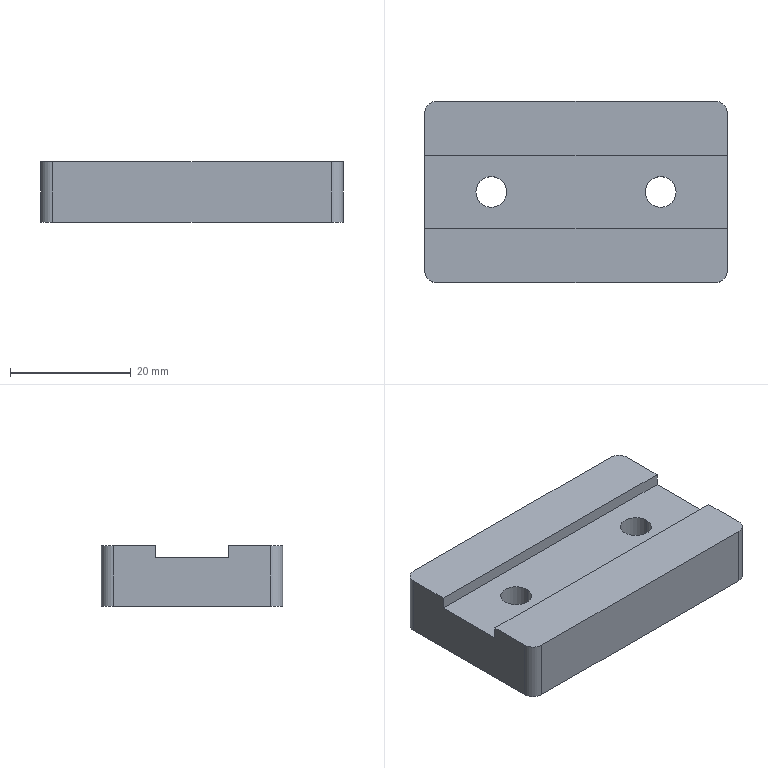Part | STEP file | PN_0044 | 1 solid | 18 faces | box 50 x 30 x 10 mm | volume 13429 mm3 | plane 10 | cylinder 8 | commonest cylinder face diameters 4 x4 5.1 x4
STEP:
#1=CARTESIAN_POINT('',(0.,0.,0.));
#2=DIRECTION('',(0.,0.,1.));
#3=DIRECTION('',(1.,0.,0.));
#4=AXIS2_PLACEMENT_3D('',#1,#2,#3);
#5=CARTESIAN_POINT('',(16.55,0.,0.));
#6=VERTEX_POINT('',#5);
#7=CARTESIAN_POINT('',(16.55,0.,8.));
#8=VERTEX_POINT('',#7);
#9=CARTESIAN_POINT('',(16.55,0.,-7.212));
#10=DIRECTION('',(0.,0.,1.));
#11=VECTOR('',#10,1.);
#12=LINE('',#9,#11);
#13=CARTESIAN_POINT('',(14.,0.,-7.212));
#14=DIRECTION('',(0.,0.,1.));
#15=DIRECTION('',(1.,0.,0.));
#16=AXIS2_PLACEMENT_3D('',#13,#14,#15);
#17=CYLINDRICAL_SURFACE('',#16,2.55);
#18=CARTESIAN_POINT('',(6.283,0.));
#19=DIRECTION('',(0.,1.));
#20=VECTOR('',#19,1.);
#21=LINE('',#18,#20);
#22=(GEOMETRIC_REPRESENTATION_CONTEXT(2)PARAMETRIC_REPRESENTATION_CONTEXT()REPRESENTATION_CONTEXT('',''));
#23=DEFINITIONAL_REPRESENTATION('',(#21),#22);
#24=PCURVE('',#17,#23);
#25=CARTESIAN_POINT('',(14.,0.,-7.212));
#26=DIRECTION('',(0.,0.,1.));
#27=DIRECTION('',(1.,0.,0.));
#28=AXIS2_PLACEMENT_3D('',#25,#26,#27);
#29=CYLINDRICAL_SURFACE('',#28,2.55);
#30=CARTESIAN_POINT('',(0.,0.));
#31=DIRECTION('',(0.,1.));
#32=VECTOR('',#31,1.);
#33=LINE('',#30,#32);
#34=(GEOMETRIC_REPRESENTATION_CONTEXT(2)PARAMETRIC_REPRESENTATION_CONTEXT()REPRESENTATION_CONTEXT('',''));
#35=DEFINITIONAL_REPRESENTATION('',(#33),#34);
#36=PCURVE('',#29,#35);
#37=SURFACE_CURVE('',#12,(#24,#36),.PCURVE_S1.);
#38=EDGE_CURVE('',#6,#8,#37,.T.);
#39=ORIENTED_EDGE('',*,*,#38,.T.);
#40=CARTESIAN_POINT('',(11.45,0.,8.));
#41=VERTEX_POINT('',#40);
#42=CARTESIAN_POINT('',(14.,0.,8.));
#43=DIRECTION('',(0.,0.,1.));
#44=DIRECTION('',(1.,0.,0.));
#45=AXIS2_PLACEMENT_3D('',#42,#43,#44);
#46=CIRCLE('',#45,2.55);
#47=CARTESIAN_POINT('',(0.,15.212));
#48=DIRECTION('',(1.,0.));
#49=VECTOR('',#48,1.);
#50=LINE('',#47,#49);
#51=(GEOMETRIC_REPRESENTATION_CONTEXT(2)PARAMETRIC_REPRESENTATION_CONTEXT()REPRESENTATION_CONTEXT('',''));
#52=DEFINITIONAL_REPRESENTATION('',(#50),#51);
#53=PCURVE('',#17,#52);
#54=CARTESIAN_POINT('',(0.,0.,8.));
#55=DIRECTION('',(0.,0.,-1.));
#56=DIRECTION('',(-1.,0.,0.));
#57=AXIS2_PLACEMENT_3D('',#54,#55,#56);
#58=PLANE('',#57);
#59=CARTESIAN_POINT('',(-16.55,0.));
#60=CARTESIAN_POINT('',(-16.55,4.417));
#61=CARTESIAN_POINT('',(-12.725,2.208));
#62=CARTESIAN_POINT('',(-8.9,0.));
#63=CARTESIAN_POINT('',(-12.725,-2.208));
#64=CARTESIAN_POINT('',(-16.55,-4.417));
#65=CARTESIAN_POINT('',(-16.55,0.));
#66=(BOUNDED_CURVE()B_SPLINE_CURVE(2,(#59,#60,#61,#62,#63,#64,#65),.UNSPECIFIED.,.T.,.F.)B_SPLINE_CURVE_WITH_KNOTS((1,2,2,2,2,1),(-2.094,0.,2.094,4.189,6.283,8.378),.UNSPECIFIED.)CURVE()GEOMETRIC_REPRESENTATION_ITEM()RATIONAL_B_SPLINE_CURVE((1.,0.5,1.,0.5,1.,0.5,1.))REPRESENTATION_ITEM(''));
#67=(GEOMETRIC_REPRESENTATION_CONTEXT(2)PARAMETRIC_REPRESENTATION_CONTEXT()REPRESENTATION_CONTEXT('',''));
#68=DEFINITIONAL_REPRESENTATION('',(#66),#67);
#69=PCURVE('',#58,#68);
#70=SURFACE_CURVE('',#46,(#53,#69),.PCURVE_S1.);
#71=EDGE_CURVE('',#41,#8,#70,.T.);
#72=ORIENTED_EDGE('',*,*,#71,.F.);
#73=CARTESIAN_POINT('',(11.45,0.,0.));
#74=VERTEX_POINT('',#73);
#75=CARTESIAN_POINT('',(11.45,0.,-7.212));
#76=DIRECTION('',(0.,0.,1.));
#77=VECTOR('',#76,1.);
#78=LINE('',#75,#77);
#79=CARTESIAN_POINT('',(3.142,0.));
#80=DIRECTION('',(0.,1.));
#81=VECTOR('',#80,1.);
#82=LINE('',#79,#81);
#83=(GEOMETRIC_REPRESENTATION_CONTEXT(2)PARAMETRIC_REPRESENTATION_CONTEXT()REPRESENTATION_CONTEXT('',''));
#84=DEFINITIONAL_REPRESENTATION('',(#82),#83);
#85=PCURVE('',#17,#84);
#86=CARTESIAN_POINT('',(3.142,0.));
#87=DIRECTION('',(0.,1.));
#88=VECTOR('',#87,1.);
#89=LINE('',#86,#88);
#90=(GEOMETRIC_REPRESENTATION_CONTEXT(2)PARAMETRIC_REPRESENTATION_CONTEXT()REPRESENTATION_CONTEXT('',''));
#91=DEFINITIONAL_REPRESENTATION('',(#89),#90);
#92=PCURVE('',#29,#91);
#93=SURFACE_CURVE('',#78,(#85,#92),.PCURVE_S1.);
#94=EDGE_CURVE('',#74,#41,#93,.T.);
#95=ORIENTED_EDGE('',*,*,#94,.F.);
#96=CARTESIAN_POINT('',(14.,0.,0.));
#97=DIRECTION('',(0.,0.,1.));
#98=DIRECTION('',(-1.,0.,0.));
#99=AXIS2_PLACEMENT_3D('',#96,#97,#98);
#100=CIRCLE('',#99,2.55);
#101=CARTESIAN_POINT('',(3.142,7.212));
#102=DIRECTION('',(1.,0.));
#103=VECTOR('',#102,1.);
#104=LINE('',#101,#103);
#105=(GEOMETRIC_REPRESENTATION_CONTEXT(2)PARAMETRIC_REPRESENTATION_CONTEXT()REPRESENTATION_CONTEXT('',''));
#106=DEFINITIONAL_REPRESENTATION('',(#104),#105);
#107=PCURVE('',#17,#106);
#108=CARTESIAN_POINT('',(0.,0.,0.));
#109=DIRECTION('',(0.,0.,-1.));
#110=DIRECTION('',(-1.,0.,0.));
#111=AXIS2_PLACEMENT_3D('',#108,#109,#110);
#112=PLANE('',#111);
#113=CARTESIAN_POINT('',(-11.45,0.));
#114=CARTESIAN_POINT('',(-11.45,-4.417));
#115=CARTESIAN_POINT('',(-15.275,-2.208));
#116=CARTESIAN_POINT('',(-19.1,0.));
#117=CARTESIAN_POINT('',(-15.275,2.208));
#118=CARTESIAN_POINT('',(-11.45,4.417));
#119=CARTESIAN_POINT('',(-11.45,0.));
#120=(BOUNDED_CURVE()B_SPLINE_CURVE(2,(#113,#114,#115,#116,#117,#118,#119),.UNSPECIFIED.,.T.,.F.)B_SPLINE_CURVE_WITH_KNOTS((1,2,2,2,2,1),(-2.094,0.,2.094,4.189,6.283,8.378),.UNSPECIFIED.)CURVE()GEOMETRIC_REPRESENTATION_ITEM()RATIONAL_B_SPLINE_CURVE((1.,0.5,1.,0.5,1.,0.5,1.))REPRESENTATION_ITEM(''));
#121=(GEOMETRIC_REPRESENTATION_CONTEXT(2)PARAMETRIC_REPRESENTATION_CONTEXT()REPRESENTATION_CONTEXT('',''));
#122=DEFINITIONAL_REPRESENTATION('',(#120),#121);
#123=PCURVE('',#112,#122);
#124=SURFACE_CURVE('',#100,(#107,#123),.PCURVE_S1.);
#125=EDGE_CURVE('',#74,#6,#124,.T.);
#126=ORIENTED_EDGE('',*,*,#125,.T.);
#127=EDGE_LOOP('',(#39,#72,#95,#126));
#128=FACE_BOUND('',#127,.F.);
#129=ADVANCED_FACE('',(#128),#17,.F.);
#130=CARTESIAN_POINT('',(-11.45,0.,0.));
#131=VERTEX_POINT('',#130);
#132=CARTESIAN_POINT('',(-11.45,0.,8.));
#133=VERTEX_POINT('',#132);
#134=CARTESIAN_POINT('',(-11.45,0.,-7.212));
#135=DIRECTION('',(0.,0.,1.));
#136=VECTOR('',#135,1.);
#137=LINE('',#134,#136);
#138=CARTESIAN_POINT('',(-14.,0.,-7.212));
#139=DIRECTION('',(0.,0.,1.));
#140=DIRECTION('',(1.,0.,0.));
#141=AXIS2_PLACEMENT_3D('',#138,#139,#140);
#142=CYLINDRICAL_SURFACE('',#141,2.55);
#143=CARTESIAN_POINT('',(6.283,0.));
#144=DIRECTION('',(0.,1.));
#145=VECTOR('',#144,1.);
#146=LINE('',#143,#145);
#147=(GEOMETRIC_REPRESENTATION_CONTEXT(2)PARAMETRIC_REPRESENTATION_CONTEXT()REPRESENTATION_CONTEXT('',''));
#148=DEFINITIONAL_REPRESENTATION('',(#146),#147);
#149=PCURVE('',#142,#148);
#150=CARTESIAN_POINT('',(-14.,0.,-7.212));
#151=DIRECTION('',(0.,0.,1.));
#152=DIRECTION('',(1.,0.,0.));
#153=AXIS2_PLACEMENT_3D('',#150,#151,#152);
#154=CYLINDRICAL_SURFACE('',#153,2.55);
#155=CARTESIAN_POINT('',(0.,0.));
#156=DIRECTION('',(0.,1.));
#157=VECTOR('',#156,1.);
#158=LINE('',#155,#157);
#159=(GEOMETRIC_REPRESENTATION_CONTEXT(2)PARAMETRIC_REPRESENTATION_CONTEXT()REPRESENTATION_CONTEXT('',''));
#160=DEFINITIONAL_REPRESENTATION('',(#158),#159);
#161=PCURVE('',#154,#160);
#162=SURFACE_CURVE('',#137,(#149,#161),.PCURVE_S1.);
#163=EDGE_CURVE('',#131,#133,#162,.T.);
#164=ORIENTED_EDGE('',*,*,#163,.T.);
#165=CARTESIAN_POINT('',(-16.55,0.,8.));
#166=VERTEX_POINT('',#165);
#167=CARTESIAN_POINT('',(-14.,0.,8.));
#168=DIRECTION('',(0.,0.,1.));
#169=DIRECTION('',(1.,0.,0.));
#170=AXIS2_PLACEMENT_3D('',#167,#168,#169);
#171=CIRCLE('',#170,2.55);
#172=CARTESIAN_POINT('',(0.,15.212));
#173=DIRECTION('',(1.,0.));
#174=VECTOR('',#173,1.);
#175=LINE('',#172,#174);
#176=(GEOMETRIC_REPRESENTATION_CONTEXT(2)PARAMETRIC_REPRESENTATION_CONTEXT()REPRESENTATION_CONTEXT('',''));
#177=DEFINITIONAL_REPRESENTATION('',(#175),#176);
#178=PCURVE('',#142,#177);
#179=CARTESIAN_POINT('',(11.45,0.));
#180=CARTESIAN_POINT('',(11.45,4.417));
#181=CARTESIAN_POINT('',(15.275,2.208));
#182=CARTESIAN_POINT('',(19.1,0.));
#183=CARTESIAN_POINT('',(15.275,-2.208));
#184=CARTESIAN_POINT('',(11.45,-4.417));
#185=CARTESIAN_POINT('',(11.45,0.));
#186=(BOUNDED_CURVE()B_SPLINE_CURVE(2,(#179,#180,#181,#182,#183,#184,#185),.UNSPECIFIED.,.T.,.F.)B_SPLINE_CURVE_WITH_KNOTS((1,2,2,2,2,1),(-2.094,0.,2.094,4.189,6.283,8.378),.UNSPECIFIED.)CURVE()GEOMETRIC_REPRESENTATION_ITEM()RATIONAL_B_SPLINE_CURVE((1.,0.5,1.,0.5,1.,0.5,1.))REPRESENTATION_ITEM(''));
#187=(GEOMETRIC_REPRESENTATION_CONTEXT(2)PARAMETRIC_REPRESENTATION_CONTEXT()REPRESENTATION_CONTEXT('',''));
#188=DEFINITIONAL_REPRESENTATION('',(#186),#187);
#189=PCURVE('',#58,#188);
#190=SURFACE_CURVE('',#171,(#178,#189),.PCURVE_S1.);
#191=EDGE_CURVE('',#166,#133,#190,.T.);
#192=ORIENTED_EDGE('',*,*,#191,.F.);
#193=CARTESIAN_POINT('',(-16.55,0.,0.));
#194=VERTEX_POINT('',#193);
#195=CARTESIAN_POINT('',(-16.55,0.,-7.212));
#196=DIRECTION('',(0.,0.,1.));
#197=VECTOR('',#196,1.);
#198=LINE('',#195,#197);
#199=CARTESIAN_POINT('',(3.142,0.));
#200=DIRECTION('',(0.,1.));
#201=VECTOR('',#200,1.);
#202=LINE('',#199,#201);
#203=(GEOMETRIC_REPRESENTATION_CONTEXT(2)PARAMETRIC_REPRESENTATION_CONTEXT()REPRESENTATION_CONTEXT('',''));
#204=DEFINITIONAL_REPRESENTATION('',(#202),#203);
#205=PCURVE('',#142,#204);
#206=CARTESIAN_POINT('',(3.142,0.));
#207=DIRECTION('',(0.,1.));
#208=VECTOR('',#207,1.);
#209=LINE('',#206,#208);
#210=(GEOMETRIC_REPRESENTATION_CONTEXT(2)PARAMETRIC_REPRESENTATION_CONTEXT()REPRESENTATION_CONTEXT('',''));
#211=DEFINITIONAL_REPRESENTATION('',(#209),#210);
#212=PCURVE('',#154,#211);
#213=SURFACE_CURVE('',#198,(#205,#212),.PCURVE_S1.);
#214=EDGE_CURVE('',#194,#166,#213,.T.);
#215=ORIENTED_EDGE('',*,*,#214,.F.);
#216=CARTESIAN_POINT('',(-14.,0.,0.));
#217=DIRECTION('',(0.,0.,1.));
#218=DIRECTION('',(-1.,0.,0.));
#219=AXIS2_PLACEMENT_3D('',#216,#217,#218);
#220=CIRCLE('',#219,2.55);
#221=CARTESIAN_POINT('',(3.142,7.212));
#222=DIRECTION('',(1.,0.));
#223=VECTOR('',#222,1.);
#224=LINE('',#221,#223);
#225=(GEOMETRIC_REPRESENTATION_CONTEXT(2)PARAMETRIC_REPRESENTATION_CONTEXT()REPRESENTATION_CONTEXT('',''));
#226=DEFINITIONAL_REPRESENTATION('',(#224),#225);
#227=PCURVE('',#142,#226);
#228=CARTESIAN_POINT('',(16.55,0.));
#229=CARTESIAN_POINT('',(16.55,-4.417));
#230=CARTESIAN_POINT('',(12.725,-2.208));
#231=CARTESIAN_POINT('',(8.9,0.));
#232=CARTESIAN_POINT('',(12.725,2.208));
#233=CARTESIAN_POINT('',(16.55,4.417));
#234=CARTESIAN_POINT('',(16.55,0.));
#235=(BOUNDED_CURVE()B_SPLINE_CURVE(2,(#228,#229,#230,#231,#232,#233,#234),.UNSPECIFIED.,.T.,.F.)B_SPLINE_CURVE_WITH_KNOTS((1,2,2,2,2,1),(-2.094,0.,2.094,4.189,6.283,8.378),.UNSPECIFIED.)CURVE()GEOMETRIC_REPRESENTATION_ITEM()RATIONAL_B_SPLINE_CURVE((1.,0.5,1.,0.5,1.,0.5,1.))REPRESENTATION_ITEM(''));
#236=(GEOMETRIC_REPRESENTATION_CONTEXT(2)PARAMETRIC_REPRESENTATION_CONTEXT()REPRESENTATION_CONTEXT('',''));
#237=DEFINITIONAL_REPRESENTATION('',(#235),#236);
#238=PCURVE('',#112,#237);
#239=SURFACE_CURVE('',#220,(#227,#238),.PCURVE_S1.);
#240=EDGE_CURVE('',#194,#131,#239,.T.);
#241=ORIENTED_EDGE('',*,*,#240,.T.);
#242=EDGE_LOOP('',(#164,#192,#215,#241));
#243=FACE_BOUND('',#242,.F.);
#244=ADVANCED_FACE('',(#243),#142,.F.);
#245=CARTESIAN_POINT('',(-25.,-6.05,10.));
#246=VERTEX_POINT('',#245);
#247=CARTESIAN_POINT('',(-25.,-13.,10.));
#248=VERTEX_POINT('',#247);
#249=CARTESIAN_POINT('',(-25.,-15.,10.));
#250=DIRECTION('',(0.,-1.,0.));
#251=VECTOR('',#250,1.);
#252=LINE('',#249,#251);
#253=CARTESIAN_POINT('',(0.,0.,10.));
#254=DIRECTION('',(0.,0.,-1.));
#255=DIRECTION('',(-1.,0.,0.));
#256=AXIS2_PLACEMENT_3D('',#253,#254,#255);
#257=PLANE('',#256);
#258=CARTESIAN_POINT('',(25.,-15.));
#259=DIRECTION('',(0.,-1.));
#260=VECTOR('',#259,1.);
#261=LINE('',#258,#260);
#262=(GEOMETRIC_REPRESENTATION_CONTEXT(2)PARAMETRIC_REPRESENTATION_CONTEXT()REPRESENTATION_CONTEXT('',''));
#263=DEFINITIONAL_REPRESENTATION('',(#261),#262);
#264=PCURVE('',#257,#263);
#265=CARTESIAN_POINT('',(-25.,-15.,10.));
#266=DIRECTION('',(1.,0.,0.));
#267=DIRECTION('',(0.,0.,-1.));
#268=AXIS2_PLACEMENT_3D('',#265,#266,#267);
#269=PLANE('',#268);
#270=CARTESIAN_POINT('',(0.,0.));
#271=DIRECTION('',(0.,-1.));
#272=VECTOR('',#271,1.);
#273=LINE('',#270,#272);
#274=(GEOMETRIC_REPRESENTATION_CONTEXT(2)PARAMETRIC_REPRESENTATION_CONTEXT()REPRESENTATION_CONTEXT('',''));
#275=DEFINITIONAL_REPRESENTATION('',(#273),#274);
#276=PCURVE('',#269,#275);
#277=SURFACE_CURVE('',#252,(#264,#276),.PCURVE_S1.);
#278=EDGE_CURVE('',#246,#248,#277,.T.);
#279=ORIENTED_EDGE('',*,*,#278,.T.);
#280=CARTESIAN_POINT('',(-23.,-15.,10.));
#281=VERTEX_POINT('',#280);
#282=CARTESIAN_POINT('',(-23.,-13.,10.));
#283=DIRECTION('',(0.,0.,1.));
#284=DIRECTION('',(-1.,0.,0.));
#285=AXIS2_PLACEMENT_3D('',#282,#283,#284);
#286=CIRCLE('',#285,2.);
#287=CARTESIAN_POINT('',(25.,-13.));
#288=CARTESIAN_POINT('',(25.,-16.464));
#289=CARTESIAN_POINT('',(22.,-14.732));
#290=CARTESIAN_POINT('',(19.,-13.));
#291=CARTESIAN_POINT('',(22.,-11.268));
#292=CARTESIAN_POINT('',(25.,-9.536));
#293=CARTESIAN_POINT('',(25.,-13.));
#294=(BOUNDED_CURVE()B_SPLINE_CURVE(2,(#287,#288,#289,#290,#291,#292,#293),.UNSPECIFIED.,.T.,.F.)B_SPLINE_CURVE_WITH_KNOTS((1,2,2,2,2,1),(-2.094,0.,2.094,4.189,6.283,8.378),.UNSPECIFIED.)CURVE()GEOMETRIC_REPRESENTATION_ITEM()RATIONAL_B_SPLINE_CURVE((1.,0.5,1.,0.5,1.,0.5,1.))REPRESENTATION_ITEM(''));
#295=(GEOMETRIC_REPRESENTATION_CONTEXT(2)PARAMETRIC_REPRESENTATION_CONTEXT()REPRESENTATION_CONTEXT('',''));
#296=DEFINITIONAL_REPRESENTATION('',(#294),#295);
#297=PCURVE('',#257,#296);
#298=CARTESIAN_POINT('',(-23.,-13.,10.));
#299=DIRECTION('',(0.,0.,-1.));
#300=DIRECTION('',(-1.,0.,0.));
#301=AXIS2_PLACEMENT_3D('',#298,#299,#300);
#302=CYLINDRICAL_SURFACE('',#301,2.);
#303=CARTESIAN_POINT('',(6.283,0.));
#304=DIRECTION('',(-1.,0.));
#305=VECTOR('',#304,1.);
#306=LINE('',#303,#305);
#307=(GEOMETRIC_REPRESENTATION_CONTEXT(2)PARAMETRIC_REPRESENTATION_CONTEXT()REPRESENTATION_CONTEXT('',''));
#308=DEFINITIONAL_REPRESENTATION('',(#306),#307);
#309=PCURVE('',#302,#308);
#310=SURFACE_CURVE('',#286,(#297,#309),.PCURVE_S1.);
#311=EDGE_CURVE('',#248,#281,#310,.T.);
#312=ORIENTED_EDGE('',*,*,#311,.T.);
#313=CARTESIAN_POINT('',(23.,-15.,10.));
#314=VERTEX_POINT('',#313);
#315=CARTESIAN_POINT('',(-25.,-15.,10.));
#316=DIRECTION('',(1.,0.,0.));
#317=VECTOR('',#316,1.);
#318=LINE('',#315,#317);
#319=CARTESIAN_POINT('',(25.,-15.));
#320=DIRECTION('',(-1.,0.));
#321=VECTOR('',#320,1.);
#322=LINE('',#319,#321);
#323=(GEOMETRIC_REPRESENTATION_CONTEXT(2)PARAMETRIC_REPRESENTATION_CONTEXT()REPRESENTATION_CONTEXT('',''));
#324=DEFINITIONAL_REPRESENTATION('',(#322),#323);
#325=PCURVE('',#257,#324);
#326=CARTESIAN_POINT('',(-25.,-15.,10.));
#327=DIRECTION('',(0.,1.,0.));
#328=DIRECTION('',(0.,0.,1.));
#329=AXIS2_PLACEMENT_3D('',#326,#327,#328);
#330=PLANE('',#329);
#331=CARTESIAN_POINT('',(0.,0.));
#332=DIRECTION('',(0.,1.));
#333=VECTOR('',#332,1.);
#334=LINE('',#331,#333);
#335=(GEOMETRIC_REPRESENTATION_CONTEXT(2)PARAMETRIC_REPRESENTATION_CONTEXT()REPRESENTATION_CONTEXT('',''));
#336=DEFINITIONAL_REPRESENTATION('',(#334),#335);
#337=PCURVE('',#330,#336);
#338=SURFACE_CURVE('',#318,(#325,#337),.PCURVE_S1.);
#339=EDGE_CURVE('',#281,#314,#338,.T.);
#340=ORIENTED_EDGE('',*,*,#339,.T.);
#341=CARTESIAN_POINT('',(25.,-13.,10.));
#342=VERTEX_POINT('',#341);
#343=CARTESIAN_POINT('',(23.,-13.,10.));
#344=DIRECTION('',(0.,0.,1.));
#345=DIRECTION('',(-1.,0.,0.));
#346=AXIS2_PLACEMENT_3D('',#343,#344,#345);
#347=CIRCLE('',#346,2.);
#348=CARTESIAN_POINT('',(-21.,-13.));
#349=CARTESIAN_POINT('',(-21.,-16.464));
#350=CARTESIAN_POINT('',(-24.,-14.732));
#351=CARTESIAN_POINT('',(-27.,-13.));
#352=CARTESIAN_POINT('',(-24.,-11.268));
#353=CARTESIAN_POINT('',(-21.,-9.536));
#354=CARTESIAN_POINT('',(-21.,-13.));
#355=(BOUNDED_CURVE()B_SPLINE_CURVE(2,(#348,#349,#350,#351,#352,#353,#354),.UNSPECIFIED.,.T.,.F.)B_SPLINE_CURVE_WITH_KNOTS((1,2,2,2,2,1),(-2.094,0.,2.094,4.189,6.283,8.378),.UNSPECIFIED.)CURVE()GEOMETRIC_REPRESENTATION_ITEM()RATIONAL_B_SPLINE_CURVE((1.,0.5,1.,0.5,1.,0.5,1.))REPRESENTATION_ITEM(''));
#356=(GEOMETRIC_REPRESENTATION_CONTEXT(2)PARAMETRIC_REPRESENTATION_CONTEXT()REPRESENTATION_CONTEXT('',''));
#357=DEFINITIONAL_REPRESENTATION('',(#355),#356);
#358=PCURVE('',#257,#357);
#359=CARTESIAN_POINT('',(23.,-13.,10.));
#360=DIRECTION('',(0.,0.,-1.));
#361=DIRECTION('',(-1.,0.,0.));
#362=AXIS2_PLACEMENT_3D('',#359,#360,#361);
#363=CYLINDRICAL_SURFACE('',#362,2.);
#364=CARTESIAN_POINT('',(6.283,0.));
#365=DIRECTION('',(-1.,0.));
#366=VECTOR('',#365,1.);
#367=LINE('',#364,#366);
#368=(GEOMETRIC_REPRESENTATION_CONTEXT(2)PARAMETRIC_REPRESENTATION_CONTEXT()REPRESENTATION_CONTEXT('',''));
#369=DEFINITIONAL_REPRESENTATION('',(#367),#368);
#370=PCURVE('',#363,#369);
#371=SURFACE_CURVE('',#347,(#358,#370),.PCURVE_S1.);
#372=EDGE_CURVE('',#314,#342,#371,.T.);
#373=ORIENTED_EDGE('',*,*,#372,.T.);
#374=CARTESIAN_POINT('',(25.,-6.05,10.));
#375=VERTEX_POINT('',#374);
#376=CARTESIAN_POINT('',(25.,-15.,10.));
#377=DIRECTION('',(0.,1.,0.));
#378=VECTOR('',#377,1.);
#379=LINE('',#376,#378);
#380=CARTESIAN_POINT('',(-25.,-15.));
#381=DIRECTION('',(0.,1.));
#382=VECTOR('',#381,1.);
#383=LINE('',#380,#382);
#384=(GEOMETRIC_REPRESENTATION_CONTEXT(2)PARAMETRIC_REPRESENTATION_CONTEXT()REPRESENTATION_CONTEXT('',''));
#385=DEFINITIONAL_REPRESENTATION('',(#383),#384);
#386=PCURVE('',#257,#385);
#387=CARTESIAN_POINT('',(25.,-15.,10.));
#388=DIRECTION('',(-1.,0.,0.));
#389=DIRECTION('',(0.,0.,1.));
#390=AXIS2_PLACEMENT_3D('',#387,#388,#389);
#391=PLANE('',#390);
#392=CARTESIAN_POINT('',(0.,0.));
#393=DIRECTION('',(0.,1.));
#394=VECTOR('',#393,1.);
#395=LINE('',#392,#394);
#396=(GEOMETRIC_REPRESENTATION_CONTEXT(2)PARAMETRIC_REPRESENTATION_CONTEXT()REPRESENTATION_CONTEXT('',''));
#397=DEFINITIONAL_REPRESENTATION('',(#395),#396);
#398=PCURVE('',#391,#397);
#399=SURFACE_CURVE('',#379,(#386,#398),.PCURVE_S1.);
#400=EDGE_CURVE('',#342,#375,#399,.T.);
#401=ORIENTED_EDGE('',*,*,#400,.T.);
#402=CARTESIAN_POINT('',(0.,-6.05,10.));
#403=DIRECTION('',(-1.,0.,0.));
#404=VECTOR('',#403,1.);
#405=LINE('',#402,#404);
#406=CARTESIAN_POINT('',(0.,-6.05));
#407=DIRECTION('',(1.,0.));
#408=VECTOR('',#407,1.);
#409=LINE('',#406,#408);
#410=(GEOMETRIC_REPRESENTATION_CONTEXT(2)PARAMETRIC_REPRESENTATION_CONTEXT()REPRESENTATION_CONTEXT('',''));
#411=DEFINITIONAL_REPRESENTATION('',(#409),#410);
#412=PCURVE('',#257,#411);
#413=CARTESIAN_POINT('',(-30.,-6.05,8.));
#414=DIRECTION('',(0.,-1.,0.));
#415=DIRECTION('',(0.,0.,-1.));
#416=AXIS2_PLACEMENT_3D('',#413,#414,#415);
#417=PLANE('',#416);
#418=CARTESIAN_POINT('',(-2.,30.));
#419=DIRECTION('',(0.,-1.));
#420=VECTOR('',#419,1.);
#421=LINE('',#418,#420);
#422=(GEOMETRIC_REPRESENTATION_CONTEXT(2)PARAMETRIC_REPRESENTATION_CONTEXT()REPRESENTATION_CONTEXT('',''));
#423=DEFINITIONAL_REPRESENTATION('',(#421),#422);
#424=PCURVE('',#417,#423);
#425=SURFACE_CURVE('',#405,(#412,#424),.PCURVE_S1.);
#426=EDGE_CURVE('',#375,#246,#425,.T.);
#427=ORIENTED_EDGE('',*,*,#426,.T.);
#428=EDGE_LOOP('',(#279,#312,#340,#373,#401,#427));
#429=FACE_BOUND('',#428,.T.);
#430=ADVANCED_FACE('',(#429),#257,.F.);
#431=ORIENTED_EDGE('',*,*,#400,.F.);
#432=CARTESIAN_POINT('',(25.,-13.,0.));
#433=VERTEX_POINT('',#432);
#434=CARTESIAN_POINT('',(25.,-13.,10.));
#435=DIRECTION('',(0.,0.,-1.));
#436=VECTOR('',#435,1.);
#437=LINE('',#434,#436);
#438=CARTESIAN_POINT('',(0.,2.));
#439=DIRECTION('',(-1.,0.));
#440=VECTOR('',#439,1.);
#441=LINE('',#438,#440);
#442=(GEOMETRIC_REPRESENTATION_CONTEXT(2)PARAMETRIC_REPRESENTATION_CONTEXT()REPRESENTATION_CONTEXT('',''));
#443=DEFINITIONAL_REPRESENTATION('',(#441),#442);
#444=PCURVE('',#391,#443);
#445=CARTESIAN_POINT('',(3.142,0.));
#446=DIRECTION('',(0.,1.));
#447=VECTOR('',#446,1.);
#448=LINE('',#445,#447);
#449=(GEOMETRIC_REPRESENTATION_CONTEXT(2)PARAMETRIC_REPRESENTATION_CONTEXT()REPRESENTATION_CONTEXT('',''));
#450=DEFINITIONAL_REPRESENTATION('',(#448),#449);
#451=PCURVE('',#363,#450);
#452=SURFACE_CURVE('',#437,(#444,#451),.PCURVE_S1.);
#453=EDGE_CURVE('',#342,#433,#452,.T.);
#454=ORIENTED_EDGE('',*,*,#453,.T.);
#455=CARTESIAN_POINT('',(25.,13.,0.));
#456=VERTEX_POINT('',#455);
#457=CARTESIAN_POINT('',(25.,-15.,0.));
#458=DIRECTION('',(0.,1.,0.));
#459=VECTOR('',#458,1.);
#460=LINE('',#457,#459);
#461=CARTESIAN_POINT('',(-10.,0.));
#462=DIRECTION('',(0.,1.));
#463=VECTOR('',#462,1.);
#464=LINE('',#461,#463);
#465=(GEOMETRIC_REPRESENTATION_CONTEXT(2)PARAMETRIC_REPRESENTATION_CONTEXT()REPRESENTATION_CONTEXT('',''));
#466=DEFINITIONAL_REPRESENTATION('',(#464),#465);
#467=PCURVE('',#391,#466);
#468=CARTESIAN_POINT('',(-25.,-15.));
#469=DIRECTION('',(0.,1.));
#470=VECTOR('',#469,1.);
#471=LINE('',#468,#470);
#472=(GEOMETRIC_REPRESENTATION_CONTEXT(2)PARAMETRIC_REPRESENTATION_CONTEXT()REPRESENTATION_CONTEXT('',''));
#473=DEFINITIONAL_REPRESENTATION('',(#471),#472);
#474=PCURVE('',#112,#473);
#475=SURFACE_CURVE('',#460,(#467,#474),.PCURVE_S1.);
#476=EDGE_CURVE('',#433,#456,#475,.T.);
#477=ORIENTED_EDGE('',*,*,#476,.T.);
#478=CARTESIAN_POINT('',(25.,13.,10.));
#479=VERTEX_POINT('',#478);
#480=CARTESIAN_POINT('',(25.,13.,10.));
#481=DIRECTION('',(0.,0.,1.));
#482=VECTOR('',#481,1.);
#483=LINE('',#480,#482);
#484=CARTESIAN_POINT('',(0.,28.));
#485=DIRECTION('',(1.,0.));
#486=VECTOR('',#485,1.);
#487=LINE('',#484,#486);
#488=(GEOMETRIC_REPRESENTATION_CONTEXT(2)PARAMETRIC_REPRESENTATION_CONTEXT()REPRESENTATION_CONTEXT('',''));
#489=DEFINITIONAL_REPRESENTATION('',(#487),#488);
#490=PCURVE('',#391,#489);
#491=CARTESIAN_POINT('',(23.,13.,10.));
#492=DIRECTION('',(0.,0.,-1.));
#493=DIRECTION('',(-1.,0.,0.));
#494=AXIS2_PLACEMENT_3D('',#491,#492,#493);
#495=CYLINDRICAL_SURFACE('',#494,2.);
#496=CARTESIAN_POINT('',(3.142,0.));
#497=DIRECTION('',(0.,-1.));
#498=VECTOR('',#497,1.);
#499=LINE('',#496,#498);
#500=(GEOMETRIC_REPRESENTATION_CONTEXT(2)PARAMETRIC_REPRESENTATION_CONTEXT()REPRESENTATION_CONTEXT('',''));
#501=DEFINITIONAL_REPRESENTATION('',(#499),#500);
#502=PCURVE('',#495,#501);
#503=SURFACE_CURVE('',#483,(#490,#502),.PCURVE_S1.);
#504=EDGE_CURVE('',#456,#479,#503,.T.);
#505=ORIENTED_EDGE('',*,*,#504,.T.);
#506=CARTESIAN_POINT('',(25.,6.05,10.));
#507=VERTEX_POINT('',#506);
#508=CARTESIAN_POINT('',(25.,-15.,10.));
#509=DIRECTION('',(0.,1.,0.));
#510=VECTOR('',#509,1.);
#511=LINE('',#508,#510);
#512=CARTESIAN_POINT('',(0.,0.));
#513=DIRECTION('',(0.,1.));
#514=VECTOR('',#513,1.);
#515=LINE('',#512,#514);
#516=(GEOMETRIC_REPRESENTATION_CONTEXT(2)PARAMETRIC_REPRESENTATION_CONTEXT()REPRESENTATION_CONTEXT('',''));
#517=DEFINITIONAL_REPRESENTATION('',(#515),#516);
#518=PCURVE('',#391,#517);
#519=CARTESIAN_POINT('',(0.,0.,10.));
#520=DIRECTION('',(0.,0.,-1.));
#521=DIRECTION('',(-1.,0.,0.));
#522=AXIS2_PLACEMENT_3D('',#519,#520,#521);
#523=PLANE('',#522);
#524=CARTESIAN_POINT('',(-25.,-15.));
#525=DIRECTION('',(0.,1.));
#526=VECTOR('',#525,1.);
#527=LINE('',#524,#526);
#528=(GEOMETRIC_REPRESENTATION_CONTEXT(2)PARAMETRIC_REPRESENTATION_CONTEXT()REPRESENTATION_CONTEXT('',''));
#529=DEFINITIONAL_REPRESENTATION('',(#527),#528);
#530=PCURVE('',#523,#529);
#531=SURFACE_CURVE('',#511,(#518,#530),.PCURVE_S1.);
#532=EDGE_CURVE('',#507,#479,#531,.T.);
#533=ORIENTED_EDGE('',*,*,#532,.F.);
#534=CARTESIAN_POINT('',(25.,6.05,8.));
#535=VERTEX_POINT('',#534);
#536=CARTESIAN_POINT('',(25.,6.05,10.));
#537=DIRECTION('',(0.,0.,-1.));
#538=VECTOR('',#537,1.);
#539=LINE('',#536,#538);
#540=CARTESIAN_POINT('',(0.,21.05));
#541=DIRECTION('',(-1.,0.));
#542=VECTOR('',#541,1.);
#543=LINE('',#540,#542);
#544=(GEOMETRIC_REPRESENTATION_CONTEXT(2)PARAMETRIC_REPRESENTATION_CONTEXT()REPRESENTATION_CONTEXT('',''));
#545=DEFINITIONAL_REPRESENTATION('',(#543),#544);
#546=PCURVE('',#391,#545);
#547=CARTESIAN_POINT('',(-30.,6.05,8.));
#548=DIRECTION('',(0.,1.,0.));
#549=DIRECTION('',(0.,0.,1.));
#550=AXIS2_PLACEMENT_3D('',#547,#548,#549);
#551=PLANE('',#550);
#552=CARTESIAN_POINT('',(2.,55.));
#553=DIRECTION('',(-1.,0.));
#554=VECTOR('',#553,1.);
#555=LINE('',#552,#554);
#556=(GEOMETRIC_REPRESENTATION_CONTEXT(2)PARAMETRIC_REPRESENTATION_CONTEXT()REPRESENTATION_CONTEXT('',''));
#557=DEFINITIONAL_REPRESENTATION('',(#555),#556);
#558=PCURVE('',#551,#557);
#559=SURFACE_CURVE('',#539,(#546,#558),.PCURVE_S1.);
#560=EDGE_CURVE('',#507,#535,#559,.T.);
#561=ORIENTED_EDGE('',*,*,#560,.T.);
#562=CARTESIAN_POINT('',(25.,-6.05,8.));
#563=VERTEX_POINT('',#562);
#564=CARTESIAN_POINT('',(25.,-15.,8.));
#565=DIRECTION('',(0.,-1.,0.));
#566=VECTOR('',#565,1.);
#567=LINE('',#564,#566);
#568=CARTESIAN_POINT('',(-2.,0.));
#569=DIRECTION('',(0.,-1.));
#570=VECTOR('',#569,1.);
#571=LINE('',#568,#570);
#572=(GEOMETRIC_REPRESENTATION_CONTEXT(2)PARAMETRIC_REPRESENTATION_CONTEXT()REPRESENTATION_CONTEXT('',''));
#573=DEFINITIONAL_REPRESENTATION('',(#571),#572);
#574=PCURVE('',#391,#573);
#575=CARTESIAN_POINT('',(-25.,-15.));
#576=DIRECTION('',(0.,-1.));
#577=VECTOR('',#576,1.);
#578=LINE('',#575,#577);
#579=(GEOMETRIC_REPRESENTATION_CONTEXT(2)PARAMETRIC_REPRESENTATION_CONTEXT()REPRESENTATION_CONTEXT('',''));
#580=DEFINITIONAL_REPRESENTATION('',(#578),#579);
#581=PCURVE('',#58,#580);
#582=SURFACE_CURVE('',#567,(#574,#581),.PCURVE_S1.);
#583=EDGE_CURVE('',#535,#563,#582,.T.);
#584=ORIENTED_EDGE('',*,*,#583,.T.);
#585=CARTESIAN_POINT('',(25.,-6.05,10.));
#586=DIRECTION('',(0.,0.,1.));
#587=VECTOR('',#586,1.);
#588=LINE('',#585,#587);
#589=CARTESIAN_POINT('',(0.,8.95));
#590=DIRECTION('',(1.,0.));
#591=VECTOR('',#590,1.);
#592=LINE('',#589,#591);
#593=(GEOMETRIC_REPRESENTATION_CONTEXT(2)PARAMETRIC_REPRESENTATION_CONTEXT()REPRESENTATION_CONTEXT('',''));
#594=DEFINITIONAL_REPRESENTATION('',(#592),#593);
#595=PCURVE('',#391,#594);
#596=CARTESIAN_POINT('',(-2.,55.));
#597=DIRECTION('',(-1.,0.));
#598=VECTOR('',#597,1.);
#599=LINE('',#596,#598);
#600=(GEOMETRIC_REPRESENTATION_CONTEXT(2)PARAMETRIC_REPRESENTATION_CONTEXT()REPRESENTATION_CONTEXT('',''));
#601=DEFINITIONAL_REPRESENTATION('',(#599),#600);
#602=PCURVE('',#417,#601);
#603=SURFACE_CURVE('',#588,(#595,#602),.PCURVE_S1.);
#604=EDGE_CURVE('',#563,#375,#603,.T.);
#605=ORIENTED_EDGE('',*,*,#604,.T.);
#606=EDGE_LOOP('',(#431,#454,#477,#505,#533,#561,#584,#605));
#607=FACE_BOUND('',#606,.T.);
#608=ADVANCED_FACE('',(#607),#391,.F.);
#609=CARTESIAN_POINT('',(23.,15.,0.));
#610=VERTEX_POINT('',#609);
#611=CARTESIAN_POINT('',(-23.,15.,0.));
#612=VERTEX_POINT('',#611);
#613=CARTESIAN_POINT('',(-25.,15.,0.));
#614=DIRECTION('',(-1.,0.,0.));
#615=VECTOR('',#614,1.);
#616=LINE('',#613,#615);
#617=CARTESIAN_POINT('',(-25.,15.,10.));
#618=DIRECTION('',(0.,-1.,0.));
#619=DIRECTION('',(0.,0.,-1.));
#620=AXIS2_PLACEMENT_3D('',#617,#618,#619);
#621=PLANE('',#620);
#622=CARTESIAN_POINT('',(10.,0.));
#623=DIRECTION('',(0.,-1.));
#624=VECTOR('',#623,1.);
#625=LINE('',#622,#624);
#626=(GEOMETRIC_REPRESENTATION_CONTEXT(2)PARAMETRIC_REPRESENTATION_CONTEXT()REPRESENTATION_CONTEXT('',''));
#627=DEFINITIONAL_REPRESENTATION('',(#625),#626);
#628=PCURVE('',#621,#627);
#629=CARTESIAN_POINT('',(25.,15.));
#630=DIRECTION('',(1.,0.));
#631=VECTOR('',#630,1.);
#632=LINE('',#629,#631);
#633=(GEOMETRIC_REPRESENTATION_CONTEXT(2)PARAMETRIC_REPRESENTATION_CONTEXT()REPRESENTATION_CONTEXT('',''));
#634=DEFINITIONAL_REPRESENTATION('',(#632),#633);
#635=PCURVE('',#112,#634);
#636=SURFACE_CURVE('',#616,(#628,#635),.PCURVE_S1.);
#637=EDGE_CURVE('',#610,#612,#636,.T.);
#638=ORIENTED_EDGE('',*,*,#637,.T.);
#639=CARTESIAN_POINT('',(-23.,15.,10.));
#640=VERTEX_POINT('',#639);
#641=CARTESIAN_POINT('',(-23.,15.,10.));
#642=DIRECTION('',(0.,0.,1.));
#643=VECTOR('',#642,1.);
#644=LINE('',#641,#643);
#645=CARTESIAN_POINT('',(0.,2.));
#646=DIRECTION('',(-1.,0.));
#647=VECTOR('',#646,1.);
#648=LINE('',#645,#647);
#649=(GEOMETRIC_REPRESENTATION_CONTEXT(2)PARAMETRIC_REPRESENTATION_CONTEXT()REPRESENTATION_CONTEXT('',''));
#650=DEFINITIONAL_REPRESENTATION('',(#648),#649);
#651=PCURVE('',#621,#650);
#652=CARTESIAN_POINT('',(-23.,13.,10.));
#653=DIRECTION('',(0.,0.,-1.));
#654=DIRECTION('',(-1.,0.,0.));
#655=AXIS2_PLACEMENT_3D('',#652,#653,#654);
#656=CYLINDRICAL_SURFACE('',#655,2.);
#657=CARTESIAN_POINT('',(1.571,0.));
#658=DIRECTION('',(0.,-1.));
#659=VECTOR('',#658,1.);
#660=LINE('',#657,#659);
#661=(GEOMETRIC_REPRESENTATION_CONTEXT(2)PARAMETRIC_REPRESENTATION_CONTEXT()REPRESENTATION_CONTEXT('',''));
#662=DEFINITIONAL_REPRESENTATION('',(#660),#661);
#663=PCURVE('',#656,#662);
#664=SURFACE_CURVE('',#644,(#651,#663),.PCURVE_S1.);
#665=EDGE_CURVE('',#612,#640,#664,.T.);
#666=ORIENTED_EDGE('',*,*,#665,.T.);
#667=CARTESIAN_POINT('',(23.,15.,10.));
#668=VERTEX_POINT('',#667);
#669=CARTESIAN_POINT('',(-25.,15.,10.));
#670=DIRECTION('',(-1.,0.,0.));
#671=VECTOR('',#670,1.);
#672=LINE('',#669,#671);
#673=CARTESIAN_POINT('',(0.,0.));
#674=DIRECTION('',(0.,-1.));
#675=VECTOR('',#674,1.);
#676=LINE('',#673,#675);
#677=(GEOMETRIC_REPRESENTATION_CONTEXT(2)PARAMETRIC_REPRESENTATION_CONTEXT()REPRESENTATION_CONTEXT('',''));
#678=DEFINITIONAL_REPRESENTATION('',(#676),#677);
#679=PCURVE('',#621,#678);
#680=CARTESIAN_POINT('',(25.,15.));
#681=DIRECTION('',(1.,0.));
#682=VECTOR('',#681,1.);
#683=LINE('',#680,#682);
#684=(GEOMETRIC_REPRESENTATION_CONTEXT(2)PARAMETRIC_REPRESENTATION_CONTEXT()REPRESENTATION_CONTEXT('',''));
#685=DEFINITIONAL_REPRESENTATION('',(#683),#684);
#686=PCURVE('',#523,#685);
#687=SURFACE_CURVE('',#672,(#679,#686),.PCURVE_S1.);
#688=EDGE_CURVE('',#668,#640,#687,.T.);
#689=ORIENTED_EDGE('',*,*,#688,.F.);
#690=CARTESIAN_POINT('',(23.,15.,10.));
#691=DIRECTION('',(0.,0.,-1.));
#692=VECTOR('',#691,1.);
#693=LINE('',#690,#692);
#694=CARTESIAN_POINT('',(0.,48.));
#695=DIRECTION('',(1.,0.));
#696=VECTOR('',#695,1.);
#697=LINE('',#694,#696);
#698=(GEOMETRIC_REPRESENTATION_CONTEXT(2)PARAMETRIC_REPRESENTATION_CONTEXT()REPRESENTATION_CONTEXT('',''));
#699=DEFINITIONAL_REPRESENTATION('',(#697),#698);
#700=PCURVE('',#621,#699);
#701=CARTESIAN_POINT('',(1.571,0.));
#702=DIRECTION('',(0.,1.));
#703=VECTOR('',#702,1.);
#704=LINE('',#701,#703);
#705=(GEOMETRIC_REPRESENTATION_CONTEXT(2)PARAMETRIC_REPRESENTATION_CONTEXT()REPRESENTATION_CONTEXT('',''));
#706=DEFINITIONAL_REPRESENTATION('',(#704),#705);
#707=PCURVE('',#495,#706);
#708=SURFACE_CURVE('',#693,(#700,#707),.PCURVE_S1.);
#709=EDGE_CURVE('',#668,#610,#708,.T.);
#710=ORIENTED_EDGE('',*,*,#709,.T.);
#711=EDGE_LOOP('',(#638,#666,#689,#710));
#712=FACE_BOUND('',#711,.T.);
#713=ADVANCED_FACE('',(#712),#621,.F.);
#714=CARTESIAN_POINT('',(-25.,13.,10.));
#715=VERTEX_POINT('',#714);
#716=CARTESIAN_POINT('',(-25.,6.05,10.));
#717=VERTEX_POINT('',#716);
#718=CARTESIAN_POINT('',(-25.,-15.,10.));
#719=DIRECTION('',(0.,-1.,0.));
#720=VECTOR('',#719,1.);
#721=LINE('',#718,#720);
#722=CARTESIAN_POINT('',(0.,0.));
#723=DIRECTION('',(0.,-1.));
#724=VECTOR('',#723,1.);
#725=LINE('',#722,#724);
#726=(GEOMETRIC_REPRESENTATION_CONTEXT(2)PARAMETRIC_REPRESENTATION_CONTEXT()REPRESENTATION_CONTEXT('',''));
#727=DEFINITIONAL_REPRESENTATION('',(#725),#726);
#728=PCURVE('',#269,#727);
#729=CARTESIAN_POINT('',(25.,-15.));
#730=DIRECTION('',(0.,-1.));
#731=VECTOR('',#730,1.);
#732=LINE('',#729,#731);
#733=(GEOMETRIC_REPRESENTATION_CONTEXT(2)PARAMETRIC_REPRESENTATION_CONTEXT()REPRESENTATION_CONTEXT('',''));
#734=DEFINITIONAL_REPRESENTATION('',(#732),#733);
#735=PCURVE('',#523,#734);
#736=SURFACE_CURVE('',#721,(#728,#735),.PCURVE_S1.);
#737=EDGE_CURVE('',#715,#717,#736,.T.);
#738=ORIENTED_EDGE('',*,*,#737,.F.);
#739=CARTESIAN_POINT('',(-25.,13.,0.));
#740=VERTEX_POINT('',#739);
#741=CARTESIAN_POINT('',(-25.,13.,10.));
#742=DIRECTION('',(0.,0.,-1.));
#743=VECTOR('',#742,1.);
#744=LINE('',#741,#743);
#745=CARTESIAN_POINT('',(0.,28.));
#746=DIRECTION('',(1.,0.));
#747=VECTOR('',#746,1.);
#748=LINE('',#745,#747);
#749=(GEOMETRIC_REPRESENTATION_CONTEXT(2)PARAMETRIC_REPRESENTATION_CONTEXT()REPRESENTATION_CONTEXT('',''));
#750=DEFINITIONAL_REPRESENTATION('',(#748),#749);
#751=PCURVE('',#269,#750);
#752=CARTESIAN_POINT('',(0.,0.));
#753=DIRECTION('',(0.,1.));
#754=VECTOR('',#753,1.);
#755=LINE('',#752,#754);
#756=(GEOMETRIC_REPRESENTATION_CONTEXT(2)PARAMETRIC_REPRESENTATION_CONTEXT()REPRESENTATION_CONTEXT('',''));
#757=DEFINITIONAL_REPRESENTATION('',(#755),#756);
#758=PCURVE('',#656,#757);
#759=SURFACE_CURVE('',#744,(#751,#758),.PCURVE_S1.);
#760=EDGE_CURVE('',#715,#740,#759,.T.);
#761=ORIENTED_EDGE('',*,*,#760,.T.);
#762=CARTESIAN_POINT('',(-25.,-13.,0.));
#763=VERTEX_POINT('',#762);
#764=CARTESIAN_POINT('',(-25.,-15.,0.));
#765=DIRECTION('',(0.,-1.,0.));
#766=VECTOR('',#765,1.);
#767=LINE('',#764,#766);
#768=CARTESIAN_POINT('',(10.,0.));
#769=DIRECTION('',(0.,-1.));
#770=VECTOR('',#769,1.);
#771=LINE('',#768,#770);
#772=(GEOMETRIC_REPRESENTATION_CONTEXT(2)PARAMETRIC_REPRESENTATION_CONTEXT()REPRESENTATION_CONTEXT('',''));
#773=DEFINITIONAL_REPRESENTATION('',(#771),#772);
#774=PCURVE('',#269,#773);
#775=CARTESIAN_POINT('',(25.,-15.));
#776=DIRECTION('',(0.,-1.));
#777=VECTOR('',#776,1.);
#778=LINE('',#775,#777);
#779=(GEOMETRIC_REPRESENTATION_CONTEXT(2)PARAMETRIC_REPRESENTATION_CONTEXT()REPRESENTATION_CONTEXT('',''));
#780=DEFINITIONAL_REPRESENTATION('',(#778),#779);
#781=PCURVE('',#112,#780);
#782=SURFACE_CURVE('',#767,(#774,#781),.PCURVE_S1.);
#783=EDGE_CURVE('',#740,#763,#782,.T.);
#784=ORIENTED_EDGE('',*,*,#783,.T.);
#785=CARTESIAN_POINT('',(-25.,-13.,10.));
#786=DIRECTION('',(0.,0.,1.));
#787=VECTOR('',#786,1.);
#788=LINE('',#785,#787);
#789=CARTESIAN_POINT('',(0.,2.));
#790=DIRECTION('',(-1.,0.));
#791=VECTOR('',#790,1.);
#792=LINE('',#789,#791);
#793=(GEOMETRIC_REPRESENTATION_CONTEXT(2)PARAMETRIC_REPRESENTATION_CONTEXT()REPRESENTATION_CONTEXT('',''));
#794=DEFINITIONAL_REPRESENTATION('',(#792),#793);
#795=PCURVE('',#269,#794);
#796=CARTESIAN_POINT('',(6.283,0.));
#797=DIRECTION('',(0.,-1.));
#798=VECTOR('',#797,1.);
#799=LINE('',#796,#798);
#800=(GEOMETRIC_REPRESENTATION_CONTEXT(2)PARAMETRIC_REPRESENTATION_CONTEXT()REPRESENTATION_CONTEXT('',''));
#801=DEFINITIONAL_REPRESENTATION('',(#799),#800);
#802=PCURVE('',#302,#801);
#803=SURFACE_CURVE('',#788,(#795,#802),.PCURVE_S1.);
#804=EDGE_CURVE('',#763,#248,#803,.T.);
#805=ORIENTED_EDGE('',*,*,#804,.T.);
#806=ORIENTED_EDGE('',*,*,#278,.F.);
#807=CARTESIAN_POINT('',(-25.,-6.05,8.));
#808=VERTEX_POINT('',#807);
#809=CARTESIAN_POINT('',(-25.,-6.05,10.));
#810=DIRECTION('',(0.,0.,-1.));
#811=VECTOR('',#810,1.);
#812=LINE('',#809,#811);
#813=CARTESIAN_POINT('',(0.,8.95));
#814=DIRECTION('',(1.,0.));
#815=VECTOR('',#814,1.);
#816=LINE('',#813,#815);
#817=(GEOMETRIC_REPRESENTATION_CONTEXT(2)PARAMETRIC_REPRESENTATION_CONTEXT()REPRESENTATION_CONTEXT('',''));
#818=DEFINITIONAL_REPRESENTATION('',(#816),#817);
#819=PCURVE('',#269,#818);
#820=CARTESIAN_POINT('',(-2.,5.));
#821=DIRECTION('',(1.,0.));
#822=VECTOR('',#821,1.);
#823=LINE('',#820,#822);
#824=(GEOMETRIC_REPRESENTATION_CONTEXT(2)PARAMETRIC_REPRESENTATION_CONTEXT()REPRESENTATION_CONTEXT('',''));
#825=DEFINITIONAL_REPRESENTATION('',(#823),#824);
#826=PCURVE('',#417,#825);
#827=SURFACE_CURVE('',#812,(#819,#826),.PCURVE_S1.);
#828=EDGE_CURVE('',#246,#808,#827,.T.);
#829=ORIENTED_EDGE('',*,*,#828,.T.);
#830=CARTESIAN_POINT('',(-25.,6.05,8.));
#831=VERTEX_POINT('',#830);
#832=CARTESIAN_POINT('',(-25.,-15.,8.));
#833=DIRECTION('',(0.,1.,0.));
#834=VECTOR('',#833,1.);
#835=LINE('',#832,#834);
#836=CARTESIAN_POINT('',(2.,0.));
#837=DIRECTION('',(0.,1.));
#838=VECTOR('',#837,1.);
#839=LINE('',#836,#838);
#840=(GEOMETRIC_REPRESENTATION_CONTEXT(2)PARAMETRIC_REPRESENTATION_CONTEXT()REPRESENTATION_CONTEXT('',''));
#841=DEFINITIONAL_REPRESENTATION('',(#839),#840);
#842=PCURVE('',#269,#841);
#843=CARTESIAN_POINT('',(25.,-15.));
#844=DIRECTION('',(0.,1.));
#845=VECTOR('',#844,1.);
#846=LINE('',#843,#845);
#847=(GEOMETRIC_REPRESENTATION_CONTEXT(2)PARAMETRIC_REPRESENTATION_CONTEXT()REPRESENTATION_CONTEXT('',''));
#848=DEFINITIONAL_REPRESENTATION('',(#846),#847);
#849=PCURVE('',#58,#848);
#850=SURFACE_CURVE('',#835,(#842,#849),.PCURVE_S1.);
#851=EDGE_CURVE('',#808,#831,#850,.T.);
#852=ORIENTED_EDGE('',*,*,#851,.T.);
#853=CARTESIAN_POINT('',(-25.,6.05,10.));
#854=DIRECTION('',(0.,0.,1.));
#855=VECTOR('',#854,1.);
#856=LINE('',#853,#855);
#857=CARTESIAN_POINT('',(0.,21.05));
#858=DIRECTION('',(-1.,0.));
#859=VECTOR('',#858,1.);
#860=LINE('',#857,#859);
#861=(GEOMETRIC_REPRESENTATION_CONTEXT(2)PARAMETRIC_REPRESENTATION_CONTEXT()REPRESENTATION_CONTEXT('',''));
#862=DEFINITIONAL_REPRESENTATION('',(#860),#861);
#863=PCURVE('',#269,#862);
#864=CARTESIAN_POINT('',(2.,5.));
#865=DIRECTION('',(1.,0.));
#866=VECTOR('',#865,1.);
#867=LINE('',#864,#866);
#868=(GEOMETRIC_REPRESENTATION_CONTEXT(2)PARAMETRIC_REPRESENTATION_CONTEXT()REPRESENTATION_CONTEXT('',''));
#869=DEFINITIONAL_REPRESENTATION('',(#867),#868);
#870=PCURVE('',#551,#869);
#871=SURFACE_CURVE('',#856,(#863,#870),.PCURVE_S1.);
#872=EDGE_CURVE('',#831,#717,#871,.T.);
#873=ORIENTED_EDGE('',*,*,#872,.T.);
#874=EDGE_LOOP('',(#738,#761,#784,#805,#806,#829,#852,#873));
#875=FACE_BOUND('',#874,.T.);
#876=ADVANCED_FACE('',(#875),#269,.F.);
#877=ORIENTED_EDGE('',*,*,#339,.F.);
#878=CARTESIAN_POINT('',(-23.,-15.,0.));
#879=VERTEX_POINT('',#878);
#880=CARTESIAN_POINT('',(-23.,-15.,10.));
#881=DIRECTION('',(0.,0.,-1.));
#882=VECTOR('',#881,1.);
#883=LINE('',#880,#882);
#884=CARTESIAN_POINT('',(0.,2.));
#885=DIRECTION('',(-1.,0.));
#886=VECTOR('',#885,1.);
#887=LINE('',#884,#886);
#888=(GEOMETRIC_REPRESENTATION_CONTEXT(2)PARAMETRIC_REPRESENTATION_CONTEXT()REPRESENTATION_CONTEXT('',''));
#889=DEFINITIONAL_REPRESENTATION('',(#887),#888);
#890=PCURVE('',#330,#889);
#891=CARTESIAN_POINT('',(4.712,0.));
#892=DIRECTION('',(0.,1.));
#893=VECTOR('',#892,1.);
#894=LINE('',#891,#893);
#895=(GEOMETRIC_REPRESENTATION_CONTEXT(2)PARAMETRIC_REPRESENTATION_CONTEXT()REPRESENTATION_CONTEXT('',''));
#896=DEFINITIONAL_REPRESENTATION('',(#894),#895);
#897=PCURVE('',#302,#896);
#898=SURFACE_CURVE('',#883,(#890,#897),.PCURVE_S1.);
#899=EDGE_CURVE('',#281,#879,#898,.T.);
#900=ORIENTED_EDGE('',*,*,#899,.T.);
#901=CARTESIAN_POINT('',(23.,-15.,0.));
#902=VERTEX_POINT('',#901);
#903=CARTESIAN_POINT('',(-25.,-15.,0.));
#904=DIRECTION('',(1.,0.,0.));
#905=VECTOR('',#904,1.);
#906=LINE('',#903,#905);
#907=CARTESIAN_POINT('',(-10.,0.));
#908=DIRECTION('',(0.,1.));
#909=VECTOR('',#908,1.);
#910=LINE('',#907,#909);
#911=(GEOMETRIC_REPRESENTATION_CONTEXT(2)PARAMETRIC_REPRESENTATION_CONTEXT()REPRESENTATION_CONTEXT('',''));
#912=DEFINITIONAL_REPRESENTATION('',(#910),#911);
#913=PCURVE('',#330,#912);
#914=CARTESIAN_POINT('',(25.,-15.));
#915=DIRECTION('',(-1.,0.));
#916=VECTOR('',#915,1.);
#917=LINE('',#914,#916);
#918=(GEOMETRIC_REPRESENTATION_CONTEXT(2)PARAMETRIC_REPRESENTATION_CONTEXT()REPRESENTATION_CONTEXT('',''));
#919=DEFINITIONAL_REPRESENTATION('',(#917),#918);
#920=PCURVE('',#112,#919);
#921=SURFACE_CURVE('',#906,(#913,#920),.PCURVE_S1.);
#922=EDGE_CURVE('',#879,#902,#921,.T.);
#923=ORIENTED_EDGE('',*,*,#922,.T.);
#924=CARTESIAN_POINT('',(23.,-15.,10.));
#925=DIRECTION('',(0.,0.,1.));
#926=VECTOR('',#925,1.);
#927=LINE('',#924,#926);
#928=CARTESIAN_POINT('',(0.,48.));
#929=DIRECTION('',(1.,0.));
#930=VECTOR('',#929,1.);
#931=LINE('',#928,#930);
#932=(GEOMETRIC_REPRESENTATION_CONTEXT(2)PARAMETRIC_REPRESENTATION_CONTEXT()REPRESENTATION_CONTEXT('',''));
#933=DEFINITIONAL_REPRESENTATION('',(#931),#932);
#934=PCURVE('',#330,#933);
#935=CARTESIAN_POINT('',(4.712,0.));
#936=DIRECTION('',(0.,-1.));
#937=VECTOR('',#936,1.);
#938=LINE('',#935,#937);
#939=(GEOMETRIC_REPRESENTATION_CONTEXT(2)PARAMETRIC_REPRESENTATION_CONTEXT()REPRESENTATION_CONTEXT('',''));
#940=DEFINITIONAL_REPRESENTATION('',(#938),#939);
#941=PCURVE('',#363,#940);
#942=SURFACE_CURVE('',#927,(#934,#941),.PCURVE_S1.);
#943=EDGE_CURVE('',#902,#314,#942,.T.);
#944=ORIENTED_EDGE('',*,*,#943,.T.);
#945=EDGE_LOOP('',(#877,#900,#923,#944));
#946=FACE_BOUND('',#945,.T.);
#947=ADVANCED_FACE('',(#946),#330,.F.);
#948=ORIENTED_EDGE('',*,*,#688,.T.);
#949=CARTESIAN_POINT('',(-23.,13.,10.));
#950=DIRECTION('',(0.,0.,1.));
#951=DIRECTION('',(-1.,0.,0.));
#952=AXIS2_PLACEMENT_3D('',#949,#950,#951);
#953=CIRCLE('',#952,2.);
#954=CARTESIAN_POINT('',(25.,13.));
#955=CARTESIAN_POINT('',(25.,9.536));
#956=CARTESIAN_POINT('',(22.,11.268));
#957=CARTESIAN_POINT('',(19.,13.));
#958=CARTESIAN_POINT('',(22.,14.732));
#959=CARTESIAN_POINT('',(25.,16.464));
#960=CARTESIAN_POINT('',(25.,13.));
#961=(BOUNDED_CURVE()B_SPLINE_CURVE(2,(#954,#955,#956,#957,#958,#959,#960),.UNSPECIFIED.,.T.,.F.)B_SPLINE_CURVE_WITH_KNOTS((1,2,2,2,2,1),(-2.094,0.,2.094,4.189,6.283,8.378),.UNSPECIFIED.)CURVE()GEOMETRIC_REPRESENTATION_ITEM()RATIONAL_B_SPLINE_CURVE((1.,0.5,1.,0.5,1.,0.5,1.))REPRESENTATION_ITEM(''));
#962=(GEOMETRIC_REPRESENTATION_CONTEXT(2)PARAMETRIC_REPRESENTATION_CONTEXT()REPRESENTATION_CONTEXT('',''));
#963=DEFINITIONAL_REPRESENTATION('',(#961),#962);
#964=PCURVE('',#523,#963);
#965=CARTESIAN_POINT('',(6.283,0.));
#966=DIRECTION('',(-1.,0.));
#967=VECTOR('',#966,1.);
#968=LINE('',#965,#967);
#969=(GEOMETRIC_REPRESENTATION_CONTEXT(2)PARAMETRIC_REPRESENTATION_CONTEXT()REPRESENTATION_CONTEXT('',''));
#970=DEFINITIONAL_REPRESENTATION('',(#968),#969);
#971=PCURVE('',#656,#970);
#972=SURFACE_CURVE('',#953,(#964,#971),.PCURVE_S1.);
#973=EDGE_CURVE('',#640,#715,#972,.T.);
#974=ORIENTED_EDGE('',*,*,#973,.T.);
#975=ORIENTED_EDGE('',*,*,#737,.T.);
#976=CARTESIAN_POINT('',(0.,6.05,10.));
#977=DIRECTION('',(1.,0.,0.));
#978=VECTOR('',#977,1.);
#979=LINE('',#976,#978);
#980=CARTESIAN_POINT('',(0.,6.05));
#981=DIRECTION('',(-1.,0.));
#982=VECTOR('',#981,1.);
#983=LINE('',#980,#982);
#984=(GEOMETRIC_REPRESENTATION_CONTEXT(2)PARAMETRIC_REPRESENTATION_CONTEXT()REPRESENTATION_CONTEXT('',''));
#985=DEFINITIONAL_REPRESENTATION('',(#983),#984);
#986=PCURVE('',#523,#985);
#987=CARTESIAN_POINT('',(2.,30.));
#988=DIRECTION('',(0.,1.));
#989=VECTOR('',#988,1.);
#990=LINE('',#987,#989);
#991=(GEOMETRIC_REPRESENTATION_CONTEXT(2)PARAMETRIC_REPRESENTATION_CONTEXT()REPRESENTATION_CONTEXT('',''));
#992=DEFINITIONAL_REPRESENTATION('',(#990),#991);
#993=PCURVE('',#551,#992);
#994=SURFACE_CURVE('',#979,(#986,#993),.PCURVE_S1.);
#995=EDGE_CURVE('',#717,#507,#994,.T.);
#996=ORIENTED_EDGE('',*,*,#995,.T.);
#997=ORIENTED_EDGE('',*,*,#532,.T.);
#998=CARTESIAN_POINT('',(23.,13.,10.));
#999=DIRECTION('',(0.,0.,1.));
#1000=DIRECTION('',(-1.,0.,0.));
#1001=AXIS2_PLACEMENT_3D('',#998,#999,#1000);
#1002=CIRCLE('',#1001,2.);
#1003=CARTESIAN_POINT('',(-21.,13.));
#1004=CARTESIAN_POINT('',(-21.,9.536));
#1005=CARTESIAN_POINT('',(-24.,11.268));
#1006=CARTESIAN_POINT('',(-27.,13.));
#1007=CARTESIAN_POINT('',(-24.,14.732));
#1008=CARTESIAN_POINT('',(-21.,16.464));
#1009=CARTESIAN_POINT('',(-21.,13.));
#1010=(BOUNDED_CURVE()B_SPLINE_CURVE(2,(#1003,#1004,#1005,#1006,#1007,#1008,#1009),.UNSPECIFIED.,.T.,.F.)B_SPLINE_CURVE_WITH_KNOTS((1,2,2,2,2,1),(-2.094,0.,2.094,4.189,6.283,8.378),.UNSPECIFIED.)CURVE()GEOMETRIC_REPRESENTATION_ITEM()RATIONAL_B_SPLINE_CURVE((1.,0.5,1.,0.5,1.,0.5,1.))REPRESENTATION_ITEM(''));
#1011=(GEOMETRIC_REPRESENTATION_CONTEXT(2)PARAMETRIC_REPRESENTATION_CONTEXT()REPRESENTATION_CONTEXT('',''));
#1012=DEFINITIONAL_REPRESENTATION('',(#1010),#1011);
#1013=PCURVE('',#523,#1012);
#1014=CARTESIAN_POINT('',(6.283,0.));
#1015=DIRECTION('',(-1.,0.));
#1016=VECTOR('',#1015,1.);
#1017=LINE('',#1014,#1016);
#1018=(GEOMETRIC_REPRESENTATION_CONTEXT(2)PARAMETRIC_REPRESENTATION_CONTEXT()REPRESENTATION_CONTEXT('',''));
#1019=DEFINITIONAL_REPRESENTATION('',(#1017),#1018);
#1020=PCURVE('',#495,#1019);
#1021=SURFACE_CURVE('',#1002,(#1013,#1020),.PCURVE_S1.);
#1022=EDGE_CURVE('',#479,#668,#1021,.T.);
#1023=ORIENTED_EDGE('',*,*,#1022,.T.);
#1024=EDGE_LOOP('',(#948,#974,#975,#996,#997,#1023));
#1025=FACE_BOUND('',#1024,.T.);
#1026=ADVANCED_FACE('',(#1025),#523,.F.);
#1027=CARTESIAN_POINT('',(14.,0.,0.));
#1028=DIRECTION('',(0.,0.,1.));
#1029=DIRECTION('',(-1.,0.,0.));
#1030=AXIS2_PLACEMENT_3D('',#1027,#1028,#1029);
#1031=CIRCLE('',#1030,2.55);
#1032=CARTESIAN_POINT('',(-11.45,0.));
#1033=CARTESIAN_POINT('',(-11.45,-4.417));
#1034=CARTESIAN_POINT('',(-15.275,-2.208));
#1035=CARTESIAN_POINT('',(-19.1,0.));
#1036=CARTESIAN_POINT('',(-15.275,2.208));
#1037=CARTESIAN_POINT('',(-11.45,4.417));
#1038=CARTESIAN_POINT('',(-11.45,0.));
#1039=(BOUNDED_CURVE()B_SPLINE_CURVE(2,(#1032,#1033,#1034,#1035,#1036,#1037,#1038),.UNSPECIFIED.,.T.,.F.)B_SPLINE_CURVE_WITH_KNOTS((1,2,2,2,2,1),(-2.094,0.,2.094,4.189,6.283,8.378),.UNSPECIFIED.)CURVE()GEOMETRIC_REPRESENTATION_ITEM()RATIONAL_B_SPLINE_CURVE((1.,0.5,1.,0.5,1.,0.5,1.))REPRESENTATION_ITEM(''));
#1040=(GEOMETRIC_REPRESENTATION_CONTEXT(2)PARAMETRIC_REPRESENTATION_CONTEXT()REPRESENTATION_CONTEXT('',''));
#1041=DEFINITIONAL_REPRESENTATION('',(#1039),#1040);
#1042=PCURVE('',#112,#1041);
#1043=CARTESIAN_POINT('',(-3.142,7.212));
#1044=DIRECTION('',(1.,0.));
#1045=VECTOR('',#1044,1.);
#1046=LINE('',#1043,#1045);
#1047=(GEOMETRIC_REPRESENTATION_CONTEXT(2)PARAMETRIC_REPRESENTATION_CONTEXT()REPRESENTATION_CONTEXT('',''));
#1048=DEFINITIONAL_REPRESENTATION('',(#1046),#1047);
#1049=PCURVE('',#29,#1048);
#1050=SURFACE_CURVE('',#1031,(#1042,#1049),.PCURVE_S1.);
#1051=EDGE_CURVE('',#6,#74,#1050,.T.);
#1052=ORIENTED_EDGE('',*,*,#1051,.T.);
#1053=ORIENTED_EDGE('',*,*,#125,.T.);
#1054=EDGE_LOOP('',(#1052,#1053));
#1055=FACE_BOUND('',#1054,.T.);
#1056=CARTESIAN_POINT('',(-14.,0.,0.));
#1057=DIRECTION('',(0.,0.,1.));
#1058=DIRECTION('',(-1.,0.,0.));
#1059=AXIS2_PLACEMENT_3D('',#1056,#1057,#1058);
#1060=CIRCLE('',#1059,2.55);
#1061=CARTESIAN_POINT('',(16.55,0.));
#1062=CARTESIAN_POINT('',(16.55,-4.417));
#1063=CARTESIAN_POINT('',(12.725,-2.208));
#1064=CARTESIAN_POINT('',(8.9,0.));
#1065=CARTESIAN_POINT('',(12.725,2.208));
#1066=CARTESIAN_POINT('',(16.55,4.417));
#1067=CARTESIAN_POINT('',(16.55,0.));
#1068=(BOUNDED_CURVE()B_SPLINE_CURVE(2,(#1061,#1062,#1063,#1064,#1065,#1066,#1067),.UNSPECIFIED.,.T.,.F.)B_SPLINE_CURVE_WITH_KNOTS((1,2,2,2,2,1),(-2.094,0.,2.094,4.189,6.283,8.378),.UNSPECIFIED.)CURVE()GEOMETRIC_REPRESENTATION_ITEM()RATIONAL_B_SPLINE_CURVE((1.,0.5,1.,0.5,1.,0.5,1.))REPRESENTATION_ITEM(''));
#1069=(GEOMETRIC_REPRESENTATION_CONTEXT(2)PARAMETRIC_REPRESENTATION_CONTEXT()REPRESENTATION_CONTEXT('',''));
#1070=DEFINITIONAL_REPRESENTATION('',(#1068),#1069);
#1071=PCURVE('',#112,#1070);
#1072=CARTESIAN_POINT('',(-3.142,7.212));
#1073=DIRECTION('',(1.,0.));
#1074=VECTOR('',#1073,1.);
#1075=LINE('',#1072,#1074);
#1076=(GEOMETRIC_REPRESENTATION_CONTEXT(2)PARAMETRIC_REPRESENTATION_CONTEXT()REPRESENTATION_CONTEXT('',''));
#1077=DEFINITIONAL_REPRESENTATION('',(#1075),#1076);
#1078=PCURVE('',#154,#1077);
#1079=SURFACE_CURVE('',#1060,(#1071,#1078),.PCURVE_S1.);
#1080=EDGE_CURVE('',#131,#194,#1079,.T.);
#1081=ORIENTED_EDGE('',*,*,#1080,.T.);
#1082=ORIENTED_EDGE('',*,*,#240,.T.);
#1083=EDGE_LOOP('',(#1081,#1082));
#1084=FACE_BOUND('',#1083,.T.);
#1085=ORIENTED_EDGE('',*,*,#783,.F.);
#1086=CARTESIAN_POINT('',(-23.,13.,0.));
#1087=DIRECTION('',(0.,0.,-1.));
#1088=DIRECTION('',(-1.,0.,0.));
#1089=AXIS2_PLACEMENT_3D('',#1086,#1087,#1088);
#1090=CIRCLE('',#1089,2.);
#1091=CARTESIAN_POINT('',(23.,13.));
#1092=DIRECTION('',(1.,0.));
#1093=AXIS2_PLACEMENT_2D('',#1091,#1092);
#1094=CIRCLE('',#1093,2.);
#1095=(GEOMETRIC_REPRESENTATION_CONTEXT(2)PARAMETRIC_REPRESENTATION_CONTEXT()REPRESENTATION_CONTEXT('',''));
#1096=DEFINITIONAL_REPRESENTATION('',(#1094),#1095);
#1097=PCURVE('',#112,#1096);
#1098=CARTESIAN_POINT('',(0.,10.));
#1099=DIRECTION('',(1.,0.));
#1100=VECTOR('',#1099,1.);
#1101=LINE('',#1098,#1100);
#1102=(GEOMETRIC_REPRESENTATION_CONTEXT(2)PARAMETRIC_REPRESENTATION_CONTEXT()REPRESENTATION_CONTEXT('',''));
#1103=DEFINITIONAL_REPRESENTATION('',(#1101),#1102);
#1104=PCURVE('',#656,#1103);
#1105=SURFACE_CURVE('',#1090,(#1097,#1104),.PCURVE_S1.);
#1106=EDGE_CURVE('',#740,#612,#1105,.T.);
#1107=ORIENTED_EDGE('',*,*,#1106,.T.);
#1108=ORIENTED_EDGE('',*,*,#637,.F.);
#1109=CARTESIAN_POINT('',(23.,13.,0.));
#1110=DIRECTION('',(0.,0.,-1.));
#1111=DIRECTION('',(-1.,0.,0.));
#1112=AXIS2_PLACEMENT_3D('',#1109,#1110,#1111);
#1113=CIRCLE('',#1112,2.);
#1114=CARTESIAN_POINT('',(-23.,13.));
#1115=DIRECTION('',(1.,0.));
#1116=AXIS2_PLACEMENT_2D('',#1114,#1115);
#1117=CIRCLE('',#1116,2.);
#1118=(GEOMETRIC_REPRESENTATION_CONTEXT(2)PARAMETRIC_REPRESENTATION_CONTEXT()REPRESENTATION_CONTEXT('',''));
#1119=DEFINITIONAL_REPRESENTATION('',(#1117),#1118);
#1120=PCURVE('',#112,#1119);
#1121=CARTESIAN_POINT('',(0.,10.));
#1122=DIRECTION('',(1.,0.));
#1123=VECTOR('',#1122,1.);
#1124=LINE('',#1121,#1123);
#1125=(GEOMETRIC_REPRESENTATION_CONTEXT(2)PARAMETRIC_REPRESENTATION_CONTEXT()REPRESENTATION_CONTEXT('',''));
#1126=DEFINITIONAL_REPRESENTATION('',(#1124),#1125);
#1127=PCURVE('',#495,#1126);
#1128=SURFACE_CURVE('',#1113,(#1120,#1127),.PCURVE_S1.);
#1129=EDGE_CURVE('',#610,#456,#1128,.T.);
#1130=ORIENTED_EDGE('',*,*,#1129,.T.);
#1131=ORIENTED_EDGE('',*,*,#476,.F.);
#1132=CARTESIAN_POINT('',(23.,-13.,0.));
#1133=DIRECTION('',(0.,0.,-1.));
#1134=DIRECTION('',(-1.,0.,0.));
#1135=AXIS2_PLACEMENT_3D('',#1132,#1133,#1134);
#1136=CIRCLE('',#1135,2.);
#1137=CARTESIAN_POINT('',(-23.,-13.));
#1138=DIRECTION('',(1.,0.));
#1139=AXIS2_PLACEMENT_2D('',#1137,#1138);
#1140=CIRCLE('',#1139,2.);
#1141=(GEOMETRIC_REPRESENTATION_CONTEXT(2)PARAMETRIC_REPRESENTATION_CONTEXT()REPRESENTATION_CONTEXT('',''));
#1142=DEFINITIONAL_REPRESENTATION('',(#1140),#1141);
#1143=PCURVE('',#112,#1142);
#1144=CARTESIAN_POINT('',(0.,10.));
#1145=DIRECTION('',(1.,0.));
#1146=VECTOR('',#1145,1.);
#1147=LINE('',#1144,#1146);
#1148=(GEOMETRIC_REPRESENTATION_CONTEXT(2)PARAMETRIC_REPRESENTATION_CONTEXT()REPRESENTATION_CONTEXT('',''));
#1149=DEFINITIONAL_REPRESENTATION('',(#1147),#1148);
#1150=PCURVE('',#363,#1149);
#1151=SURFACE_CURVE('',#1136,(#1143,#1150),.PCURVE_S1.);
#1152=EDGE_CURVE('',#433,#902,#1151,.T.);
#1153=ORIENTED_EDGE('',*,*,#1152,.T.);
#1154=ORIENTED_EDGE('',*,*,#922,.F.);
#1155=CARTESIAN_POINT('',(-23.,-13.,0.));
#1156=DIRECTION('',(0.,0.,-1.));
#1157=DIRECTION('',(-1.,0.,0.));
#1158=AXIS2_PLACEMENT_3D('',#1155,#1156,#1157);
#1159=CIRCLE('',#1158,2.);
#1160=CARTESIAN_POINT('',(23.,-13.));
#1161=DIRECTION('',(1.,0.));
#1162=AXIS2_PLACEMENT_2D('',#1160,#1161);
#1163=CIRCLE('',#1162,2.);
#1164=(GEOMETRIC_REPRESENTATION_CONTEXT(2)PARAMETRIC_REPRESENTATION_CONTEXT()REPRESENTATION_CONTEXT('',''));
#1165=DEFINITIONAL_REPRESENTATION('',(#1163),#1164);
#1166=PCURVE('',#112,#1165);
#1167=CARTESIAN_POINT('',(0.,10.));
#1168=DIRECTION('',(1.,0.));
#1169=VECTOR('',#1168,1.);
#1170=LINE('',#1167,#1169);
#1171=(GEOMETRIC_REPRESENTATION_CONTEXT(2)PARAMETRIC_REPRESENTATION_CONTEXT()REPRESENTATION_CONTEXT('',''));
#1172=DEFINITIONAL_REPRESENTATION('',(#1170),#1171);
#1173=PCURVE('',#302,#1172);
#1174=SURFACE_CURVE('',#1159,(#1166,#1173),.PCURVE_S1.);
#1175=EDGE_CURVE('',#879,#763,#1174,.T.);
#1176=ORIENTED_EDGE('',*,*,#1175,.T.);
#1177=EDGE_LOOP('',(#1085,#1107,#1108,#1130,#1131,#1153,#1154,#1176));
#1178=FACE_BOUND('',#1177,.T.);
#1179=ADVANCED_FACE('',(#1055,#1084,#1178),#112,.T.);
#1180=CARTESIAN_POINT('',(14.,0.,8.));
#1181=DIRECTION('',(0.,0.,1.));
#1182=DIRECTION('',(1.,0.,0.));
#1183=AXIS2_PLACEMENT_3D('',#1180,#1181,#1182);
#1184=CIRCLE('',#1183,2.55);
#1185=CARTESIAN_POINT('',(-16.55,0.));
#1186=CARTESIAN_POINT('',(-16.55,4.417));
#1187=CARTESIAN_POINT('',(-12.725,2.208));
#1188=CARTESIAN_POINT('',(-8.9,0.));
#1189=CARTESIAN_POINT('',(-12.725,-2.208));
#1190=CARTESIAN_POINT('',(-16.55,-4.417));
#1191=CARTESIAN_POINT('',(-16.55,0.));
#1192=(BOUNDED_CURVE()B_SPLINE_CURVE(2,(#1185,#1186,#1187,#1188,#1189,#1190,#1191),.UNSPECIFIED.,.T.,.F.)B_SPLINE_CURVE_WITH_KNOTS((1,2,2,2,2,1),(-2.094,0.,2.094,4.189,6.283,8.378),.UNSPECIFIED.)CURVE()GEOMETRIC_REPRESENTATION_ITEM()RATIONAL_B_SPLINE_CURVE((1.,0.5,1.,0.5,1.,0.5,1.))REPRESENTATION_ITEM(''));
#1193=(GEOMETRIC_REPRESENTATION_CONTEXT(2)PARAMETRIC_REPRESENTATION_CONTEXT()REPRESENTATION_CONTEXT('',''));
#1194=DEFINITIONAL_REPRESENTATION('',(#1192),#1193);
#1195=PCURVE('',#58,#1194);
#1196=CARTESIAN_POINT('',(0.,15.212));
#1197=DIRECTION('',(1.,0.));
#1198=VECTOR('',#1197,1.);
#1199=LINE('',#1196,#1198);
#1200=(GEOMETRIC_REPRESENTATION_CONTEXT(2)PARAMETRIC_REPRESENTATION_CONTEXT()REPRESENTATION_CONTEXT('',''));
#1201=DEFINITIONAL_REPRESENTATION('',(#1199),#1200);
#1202=PCURVE('',#29,#1201);
#1203=SURFACE_CURVE('',#1184,(#1195,#1202),.PCURVE_S1.);
#1204=EDGE_CURVE('',#8,#41,#1203,.T.);
#1205=ORIENTED_EDGE('',*,*,#1204,.F.);
#1206=ORIENTED_EDGE('',*,*,#71,.F.);
#1207=EDGE_LOOP('',(#1205,#1206));
#1208=FACE_BOUND('',#1207,.T.);
#1209=CARTESIAN_POINT('',(-14.,0.,8.));
#1210=DIRECTION('',(0.,0.,1.));
#1211=DIRECTION('',(1.,0.,0.));
#1212=AXIS2_PLACEMENT_3D('',#1209,#1210,#1211);
#1213=CIRCLE('',#1212,2.55);
#1214=CARTESIAN_POINT('',(11.45,0.));
#1215=CARTESIAN_POINT('',(11.45,4.417));
#1216=CARTESIAN_POINT('',(15.275,2.208));
#1217=CARTESIAN_POINT('',(19.1,0.));
#1218=CARTESIAN_POINT('',(15.275,-2.208));
#1219=CARTESIAN_POINT('',(11.45,-4.417));
#1220=CARTESIAN_POINT('',(11.45,0.));
#1221=(BOUNDED_CURVE()B_SPLINE_CURVE(2,(#1214,#1215,#1216,#1217,#1218,#1219,#1220),.UNSPECIFIED.,.T.,.F.)B_SPLINE_CURVE_WITH_KNOTS((1,2,2,2,2,1),(-2.094,0.,2.094,4.189,6.283,8.378),.UNSPECIFIED.)CURVE()GEOMETRIC_REPRESENTATION_ITEM()RATIONAL_B_SPLINE_CURVE((1.,0.5,1.,0.5,1.,0.5,1.))REPRESENTATION_ITEM(''));
#1222=(GEOMETRIC_REPRESENTATION_CONTEXT(2)PARAMETRIC_REPRESENTATION_CONTEXT()REPRESENTATION_CONTEXT('',''));
#1223=DEFINITIONAL_REPRESENTATION('',(#1221),#1222);
#1224=PCURVE('',#58,#1223);
#1225=CARTESIAN_POINT('',(0.,15.212));
#1226=DIRECTION('',(1.,0.));
#1227=VECTOR('',#1226,1.);
#1228=LINE('',#1225,#1227);
#1229=(GEOMETRIC_REPRESENTATION_CONTEXT(2)PARAMETRIC_REPRESENTATION_CONTEXT()REPRESENTATION_CONTEXT('',''));
#1230=DEFINITIONAL_REPRESENTATION('',(#1228),#1229);
#1231=PCURVE('',#154,#1230);
#1232=SURFACE_CURVE('',#1213,(#1224,#1231),.PCURVE_S1.);
#1233=EDGE_CURVE('',#133,#166,#1232,.T.);
#1234=ORIENTED_EDGE('',*,*,#1233,.F.);
#1235=ORIENTED_EDGE('',*,*,#191,.F.);
#1236=EDGE_LOOP('',(#1234,#1235));
#1237=FACE_BOUND('',#1236,.T.);
#1238=CARTESIAN_POINT('',(-30.,6.05,8.));
#1239=DIRECTION('',(-1.,0.,0.));
#1240=VECTOR('',#1239,1.);
#1241=LINE('',#1238,#1240);
#1242=CARTESIAN_POINT('',(30.,6.05));
#1243=DIRECTION('',(1.,0.));
#1244=VECTOR('',#1243,1.);
#1245=LINE('',#1242,#1244);
#1246=(GEOMETRIC_REPRESENTATION_CONTEXT(2)PARAMETRIC_REPRESENTATION_CONTEXT()REPRESENTATION_CONTEXT('',''));
#1247=DEFINITIONAL_REPRESENTATION('',(#1245),#1246);
#1248=PCURVE('',#58,#1247);
#1249=CARTESIAN_POINT('',(0.,0.));
#1250=DIRECTION('',(0.,-1.));
#1251=VECTOR('',#1250,1.);
#1252=LINE('',#1249,#1251);
#1253=(GEOMETRIC_REPRESENTATION_CONTEXT(2)PARAMETRIC_REPRESENTATION_CONTEXT()REPRESENTATION_CONTEXT('',''));
#1254=DEFINITIONAL_REPRESENTATION('',(#1252),#1253);
#1255=PCURVE('',#551,#1254);
#1256=SURFACE_CURVE('',#1241,(#1248,#1255),.PCURVE_S1.);
#1257=EDGE_CURVE('',#535,#831,#1256,.T.);
#1258=ORIENTED_EDGE('',*,*,#1257,.T.);
#1259=ORIENTED_EDGE('',*,*,#851,.F.);
#1260=CARTESIAN_POINT('',(-30.,-6.05,8.));
#1261=DIRECTION('',(1.,0.,0.));
#1262=VECTOR('',#1261,1.);
#1263=LINE('',#1260,#1262);
#1264=CARTESIAN_POINT('',(30.,-6.05));
#1265=DIRECTION('',(-1.,0.));
#1266=VECTOR('',#1265,1.);
#1267=LINE('',#1264,#1266);
#1268=(GEOMETRIC_REPRESENTATION_CONTEXT(2)PARAMETRIC_REPRESENTATION_CONTEXT()REPRESENTATION_CONTEXT('',''));
#1269=DEFINITIONAL_REPRESENTATION('',(#1267),#1268);
#1270=PCURVE('',#58,#1269);
#1271=CARTESIAN_POINT('',(0.,0.));
#1272=DIRECTION('',(0.,1.));
#1273=VECTOR('',#1272,1.);
#1274=LINE('',#1271,#1273);
#1275=(GEOMETRIC_REPRESENTATION_CONTEXT(2)PARAMETRIC_REPRESENTATION_CONTEXT()REPRESENTATION_CONTEXT('',''));
#1276=DEFINITIONAL_REPRESENTATION('',(#1274),#1275);
#1277=PCURVE('',#417,#1276);
#1278=SURFACE_CURVE('',#1263,(#1270,#1277),.PCURVE_S1.);
#1279=EDGE_CURVE('',#808,#563,#1278,.T.);
#1280=ORIENTED_EDGE('',*,*,#1279,.T.);
#1281=ORIENTED_EDGE('',*,*,#583,.F.);
#1282=EDGE_LOOP('',(#1258,#1259,#1280,#1281));
#1283=FACE_BOUND('',#1282,.T.);
#1284=ADVANCED_FACE('',(#1208,#1237,#1283),#58,.F.);
#1285=ORIENTED_EDGE('',*,*,#1279,.F.);
#1286=ORIENTED_EDGE('',*,*,#828,.F.);
#1287=ORIENTED_EDGE('',*,*,#426,.F.);
#1288=ORIENTED_EDGE('',*,*,#604,.F.);
#1289=EDGE_LOOP('',(#1285,#1286,#1287,#1288));
#1290=FACE_BOUND('',#1289,.T.);
#1291=ADVANCED_FACE('',(#1290),#417,.F.);
#1292=ORIENTED_EDGE('',*,*,#995,.F.);
#1293=ORIENTED_EDGE('',*,*,#872,.F.);
#1294=ORIENTED_EDGE('',*,*,#1257,.F.);
#1295=ORIENTED_EDGE('',*,*,#560,.F.);
#1296=EDGE_LOOP('',(#1292,#1293,#1294,#1295));
#1297=FACE_BOUND('',#1296,.T.);
#1298=ADVANCED_FACE('',(#1297),#551,.F.);
#1299=ORIENTED_EDGE('',*,*,#1233,.F.);
#1300=ORIENTED_EDGE('',*,*,#163,.F.);
#1301=ORIENTED_EDGE('',*,*,#1080,.T.);
#1302=ORIENTED_EDGE('',*,*,#214,.T.);
#1303=EDGE_LOOP('',(#1299,#1300,#1301,#1302));
#1304=FACE_BOUND('',#1303,.F.);
#1305=ADVANCED_FACE('',(#1304),#154,.F.);
#1306=ORIENTED_EDGE('',*,*,#1204,.F.);
#1307=ORIENTED_EDGE('',*,*,#38,.F.);
#1308=ORIENTED_EDGE('',*,*,#1051,.T.);
#1309=ORIENTED_EDGE('',*,*,#94,.T.);
#1310=EDGE_LOOP('',(#1306,#1307,#1308,#1309));
#1311=FACE_BOUND('',#1310,.F.);
#1312=ADVANCED_FACE('',(#1311),#29,.F.);
#1313=ORIENTED_EDGE('',*,*,#973,.F.);
#1314=ORIENTED_EDGE('',*,*,#665,.F.);
#1315=ORIENTED_EDGE('',*,*,#1106,.F.);
#1316=ORIENTED_EDGE('',*,*,#760,.F.);
#1317=EDGE_LOOP('',(#1313,#1314,#1315,#1316));
#1318=FACE_BOUND('',#1317,.T.);
#1319=ADVANCED_FACE('',(#1318),#656,.T.);
#1320=ORIENTED_EDGE('',*,*,#311,.F.);
#1321=ORIENTED_EDGE('',*,*,#804,.F.);
#1322=ORIENTED_EDGE('',*,*,#1175,.F.);
#1323=ORIENTED_EDGE('',*,*,#899,.F.);
#1324=EDGE_LOOP('',(#1320,#1321,#1322,#1323));
#1325=FACE_BOUND('',#1324,.T.);
#1326=ADVANCED_FACE('',(#1325),#302,.T.);
#1327=ORIENTED_EDGE('',*,*,#372,.F.);
#1328=ORIENTED_EDGE('',*,*,#943,.F.);
#1329=ORIENTED_EDGE('',*,*,#1152,.F.);
#1330=ORIENTED_EDGE('',*,*,#453,.F.);
#1331=EDGE_LOOP('',(#1327,#1328,#1329,#1330));
#1332=FACE_BOUND('',#1331,.T.);
#1333=ADVANCED_FACE('',(#1332),#363,.T.);
#1334=ORIENTED_EDGE('',*,*,#1022,.F.);
#1335=ORIENTED_EDGE('',*,*,#504,.F.);
#1336=ORIENTED_EDGE('',*,*,#1129,.F.);
#1337=ORIENTED_EDGE('',*,*,#709,.F.);
#1338=EDGE_LOOP('',(#1334,#1335,#1336,#1337));
#1339=FACE_BOUND('',#1338,.T.);
#1340=ADVANCED_FACE('',(#1339),#495,.T.);
#1341=CLOSED_SHELL('',(#129,#244,#430,#608,#713,#876,#947,#1026,#1179,#1284,#1291,#1298,#1305,#1312,#1319,#1326,#1333,#1340));
#1342=MANIFOLD_SOLID_BREP('',#1341);
#1343=(LENGTH_UNIT()NAMED_UNIT(*)SI_UNIT(.MILLI.,.METRE.));
#1344=UNCERTAINTY_MEASURE_WITH_UNIT(LENGTH_MEASURE(0.0000001),#1343,'','');
#1345=(NAMED_UNIT(*)PLANE_ANGLE_UNIT()SI_UNIT($,.RADIAN.));
#1346=(NAMED_UNIT(*)SI_UNIT($,.STERADIAN.)SOLID_ANGLE_UNIT());
#1347=(GEOMETRIC_REPRESENTATION_CONTEXT(3)GLOBAL_UNCERTAINTY_ASSIGNED_CONTEXT((#1344))GLOBAL_UNIT_ASSIGNED_CONTEXT((#1343,#1345,#1346))REPRESENTATION_CONTEXT('',''));
#1348=ADVANCED_BREP_SHAPE_REPRESENTATION('',(#4,#1342),#1347);